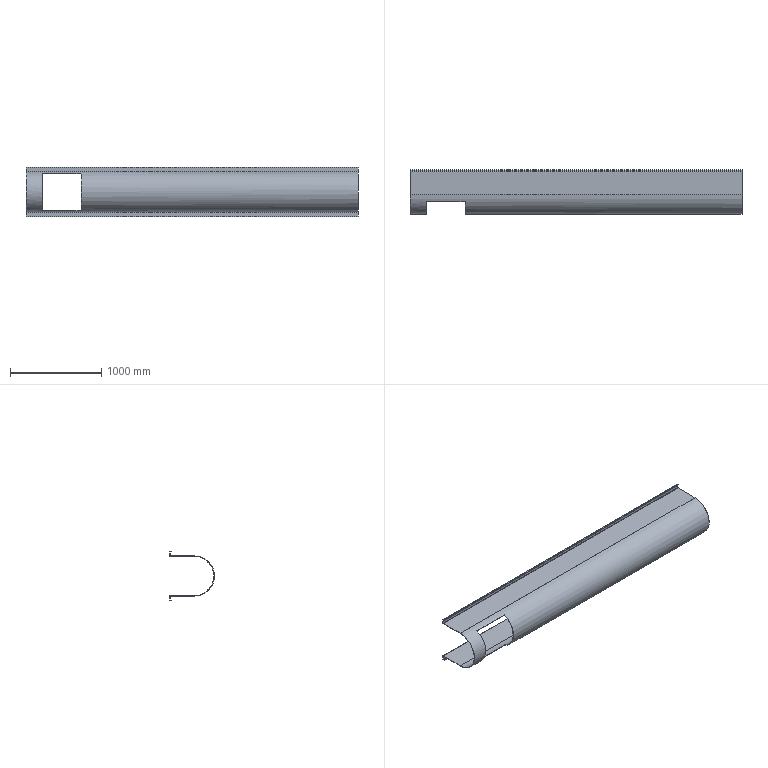Part | STEP file | Input 1 | 1 solid | 50 faces | box 3630 x 490 x 540 mm | volume 23301858 mm3 | plane 40 | cylinder 10 | commonest cylinder face diameters 5 x4 15 x4 430 x1 440 x1